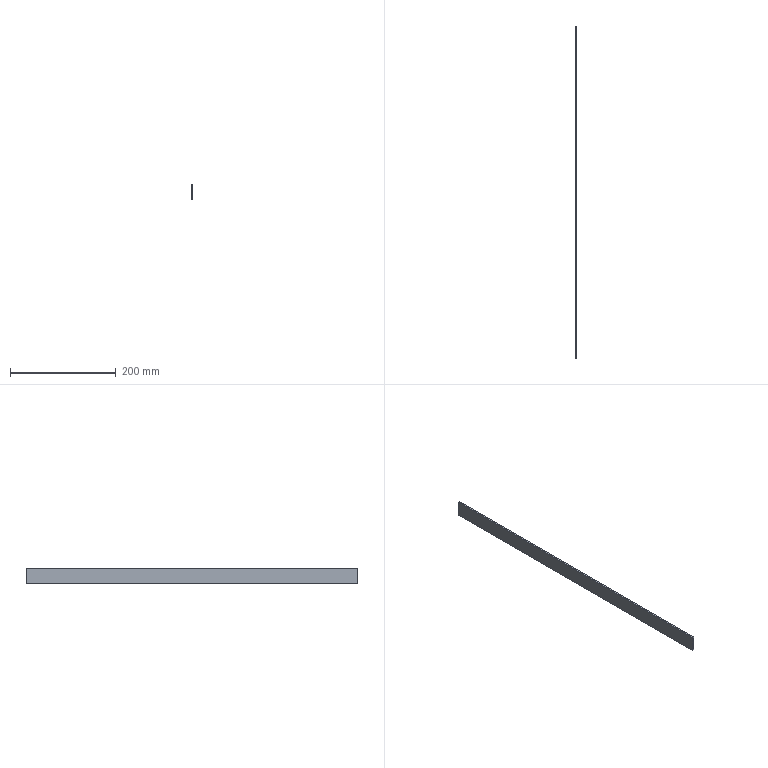Part | SolidWorks | 1 solid | 6 faces | box 3 x 628 x 30 mm | volume 56520 mm3 | plane 6
STEP:
#1=CARTESIAN_POINT('',(0.,314.,15.));
#2=VERTEX_POINT('',#1);
#3=CARTESIAN_POINT('',(0.,-314.,15.));
#4=VERTEX_POINT('',#3);
#5=CARTESIAN_POINT('',(0.,-314.,15.));
#6=DIRECTION('',(0.,-1.,0.));
#7=VECTOR('',#6,1000.);
#8=LINE('',#5,#7);
#9=EDGE_CURVE('',#2,#4,#8,.T.);
#10=ORIENTED_EDGE('',*,*,#9,.F.);
#11=CARTESIAN_POINT('',(-3.,314.,15.));
#12=VERTEX_POINT('',#11);
#13=CARTESIAN_POINT('',(-3.,314.,15.));
#14=DIRECTION('',(1.,0.,0.));
#15=VECTOR('',#14,1000.);
#16=LINE('',#13,#15);
#17=EDGE_CURVE('',#12,#2,#16,.T.);
#18=ORIENTED_EDGE('',*,*,#17,.F.);
#19=CARTESIAN_POINT('',(-3.,-314.,15.));
#20=VERTEX_POINT('',#19);
#21=CARTESIAN_POINT('',(-3.,-314.,15.));
#22=DIRECTION('',(0.,-1.,0.));
#23=VECTOR('',#22,1000.);
#24=LINE('',#21,#23);
#25=EDGE_CURVE('',#12,#20,#24,.T.);
#26=ORIENTED_EDGE('',*,*,#25,.T.);
#27=CARTESIAN_POINT('',(-3.,-314.,15.));
#28=DIRECTION('',(1.,0.,0.));
#29=VECTOR('',#28,1000.);
#30=LINE('',#27,#29);
#31=EDGE_CURVE('',#20,#4,#30,.T.);
#32=ORIENTED_EDGE('',*,*,#31,.T.);
#33=EDGE_LOOP('',(#10,#18,#26,#32));
#34=FACE_OUTER_BOUND('',#33,.T.);
#35=CARTESIAN_POINT('',(-3.,-314.,15.));
#36=DIRECTION('',(0.,0.,1.));
#37=DIRECTION('',(1.,0.,0.));
#38=AXIS2_PLACEMENT_3D('',#35,#36,#37);
#39=PLANE('',#38);
#40=ADVANCED_FACE('',(#34),#39,.T.);
#41=CARTESIAN_POINT('',(0.,314.,-15.));
#42=VERTEX_POINT('',#41);
#43=CARTESIAN_POINT('',(0.,314.,-15.));
#44=DIRECTION('',(0.,0.,1.));
#45=VECTOR('',#44,1000.);
#46=LINE('',#43,#45);
#47=EDGE_CURVE('',#42,#2,#46,.T.);
#48=ORIENTED_EDGE('',*,*,#47,.F.);
#49=CARTESIAN_POINT('',(-3.,314.,-15.));
#50=VERTEX_POINT('',#49);
#51=CARTESIAN_POINT('',(-3.,314.,-15.));
#52=DIRECTION('',(1.,0.,0.));
#53=VECTOR('',#52,1000.);
#54=LINE('',#51,#53);
#55=EDGE_CURVE('',#50,#42,#54,.T.);
#56=ORIENTED_EDGE('',*,*,#55,.F.);
#57=CARTESIAN_POINT('',(-3.,314.,-15.));
#58=DIRECTION('',(0.,0.,1.));
#59=VECTOR('',#58,1000.);
#60=LINE('',#57,#59);
#61=EDGE_CURVE('',#50,#12,#60,.T.);
#62=ORIENTED_EDGE('',*,*,#61,.T.);
#63=ORIENTED_EDGE('',*,*,#17,.T.);
#64=EDGE_LOOP('',(#48,#56,#62,#63));
#65=FACE_OUTER_BOUND('',#64,.T.);
#66=CARTESIAN_POINT('',(-3.,314.,-15.));
#67=DIRECTION('',(0.,1.,0.));
#68=DIRECTION('',(0.,0.,1.));
#69=AXIS2_PLACEMENT_3D('',#66,#67,#68);
#70=PLANE('',#69);
#71=ADVANCED_FACE('',(#65),#70,.T.);
#72=CARTESIAN_POINT('',(0.,-314.,-15.));
#73=VERTEX_POINT('',#72);
#74=CARTESIAN_POINT('',(0.,-314.,-15.));
#75=DIRECTION('',(0.,1.,0.));
#76=VECTOR('',#75,1000.);
#77=LINE('',#74,#76);
#78=EDGE_CURVE('',#73,#42,#77,.T.);
#79=ORIENTED_EDGE('',*,*,#78,.F.);
#80=CARTESIAN_POINT('',(-3.,-314.,-15.));
#81=VERTEX_POINT('',#80);
#82=CARTESIAN_POINT('',(-3.,-314.,-15.));
#83=DIRECTION('',(1.,0.,0.));
#84=VECTOR('',#83,1000.);
#85=LINE('',#82,#84);
#86=EDGE_CURVE('',#81,#73,#85,.T.);
#87=ORIENTED_EDGE('',*,*,#86,.F.);
#88=CARTESIAN_POINT('',(-3.,-314.,-15.));
#89=DIRECTION('',(0.,1.,0.));
#90=VECTOR('',#89,1000.);
#91=LINE('',#88,#90);
#92=EDGE_CURVE('',#81,#50,#91,.T.);
#93=ORIENTED_EDGE('',*,*,#92,.T.);
#94=ORIENTED_EDGE('',*,*,#55,.T.);
#95=EDGE_LOOP('',(#79,#87,#93,#94));
#96=FACE_OUTER_BOUND('',#95,.T.);
#97=CARTESIAN_POINT('',(-3.,-314.,-15.));
#98=DIRECTION('',(0.,0.,-1.));
#99=DIRECTION('',(-1.,0.,0.));
#100=AXIS2_PLACEMENT_3D('',#97,#98,#99);
#101=PLANE('',#100);
#102=ADVANCED_FACE('',(#96),#101,.T.);
#103=CARTESIAN_POINT('',(0.,-314.,-15.));
#104=DIRECTION('',(0.,0.,-1.));
#105=VECTOR('',#104,1000.);
#106=LINE('',#103,#105);
#107=EDGE_CURVE('',#4,#73,#106,.T.);
#108=ORIENTED_EDGE('',*,*,#107,.F.);
#109=ORIENTED_EDGE('',*,*,#31,.F.);
#110=CARTESIAN_POINT('',(-3.,-314.,-15.));
#111=DIRECTION('',(0.,0.,-1.));
#112=VECTOR('',#111,1000.);
#113=LINE('',#110,#112);
#114=EDGE_CURVE('',#20,#81,#113,.T.);
#115=ORIENTED_EDGE('',*,*,#114,.T.);
#116=ORIENTED_EDGE('',*,*,#86,.T.);
#117=EDGE_LOOP('',(#108,#109,#115,#116));
#118=FACE_OUTER_BOUND('',#117,.T.);
#119=CARTESIAN_POINT('',(-3.,-314.,-15.));
#120=DIRECTION('',(0.,-1.,0.));
#121=DIRECTION('',(0.,0.,-1.));
#122=AXIS2_PLACEMENT_3D('',#119,#120,#121);
#123=PLANE('',#122);
#124=ADVANCED_FACE('',(#118),#123,.T.);
#125=ORIENTED_EDGE('',*,*,#25,.F.);
#126=ORIENTED_EDGE('',*,*,#61,.F.);
#127=ORIENTED_EDGE('',*,*,#92,.F.);
#128=ORIENTED_EDGE('',*,*,#114,.F.);
#129=EDGE_LOOP('',(#125,#126,#127,#128));
#130=FACE_OUTER_BOUND('',#129,.T.);
#131=CARTESIAN_POINT('',(-3.,0.,0.));
#132=DIRECTION('',(1.,0.,0.));
#133=DIRECTION('',(0.,0.,-1.));
#134=AXIS2_PLACEMENT_3D('',#131,#132,#133);
#135=PLANE('',#134);
#136=ADVANCED_FACE('',(#130),#135,.F.);
#137=ORIENTED_EDGE('',*,*,#9,.T.);
#138=ORIENTED_EDGE('',*,*,#107,.T.);
#139=ORIENTED_EDGE('',*,*,#78,.T.);
#140=ORIENTED_EDGE('',*,*,#47,.T.);
#141=EDGE_LOOP('',(#137,#138,#139,#140));
#142=FACE_OUTER_BOUND('',#141,.T.);
#143=CARTESIAN_POINT('',(0.,0.,0.));
#144=DIRECTION('',(1.,0.,0.));
#145=DIRECTION('',(0.,0.,-1.));
#146=AXIS2_PLACEMENT_3D('',#143,#144,#145);
#147=PLANE('',#146);
#148=ADVANCED_FACE('',(#142),#147,.T.);
#149=CLOSED_SHELL('',(#40,#71,#102,#124,#136,#148));
#150=MANIFOLD_SOLID_BREP('',#149);
#151=CARTESIAN_POINT('',(0.,0.,0.));
#152=DIRECTION('',(0.,0.,1.));
#153=DIRECTION('',(1.,0.,0.));
#154=AXIS2_PLACEMENT_3D('',#151,#152,#153);
#155=(LENGTH_UNIT()NAMED_UNIT(*)SI_UNIT(.MILLI.,.METRE.));
#156=UNCERTAINTY_MEASURE_WITH_UNIT(LENGTH_MEASURE(0.00001),#155,'','');
#157=(NAMED_UNIT(*)PLANE_ANGLE_UNIT()SI_UNIT($,.RADIAN.));
#158=(NAMED_UNIT(*)SI_UNIT($,.STERADIAN.)SOLID_ANGLE_UNIT());
#159=(GEOMETRIC_REPRESENTATION_CONTEXT(3)GLOBAL_UNCERTAINTY_ASSIGNED_CONTEXT((#156))GLOBAL_UNIT_ASSIGNED_CONTEXT((#155,#157,#158))REPRESENTATION_CONTEXT('',''));
#160=ADVANCED_BREP_SHAPE_REPRESENTATION('',(#150,#154),#159);